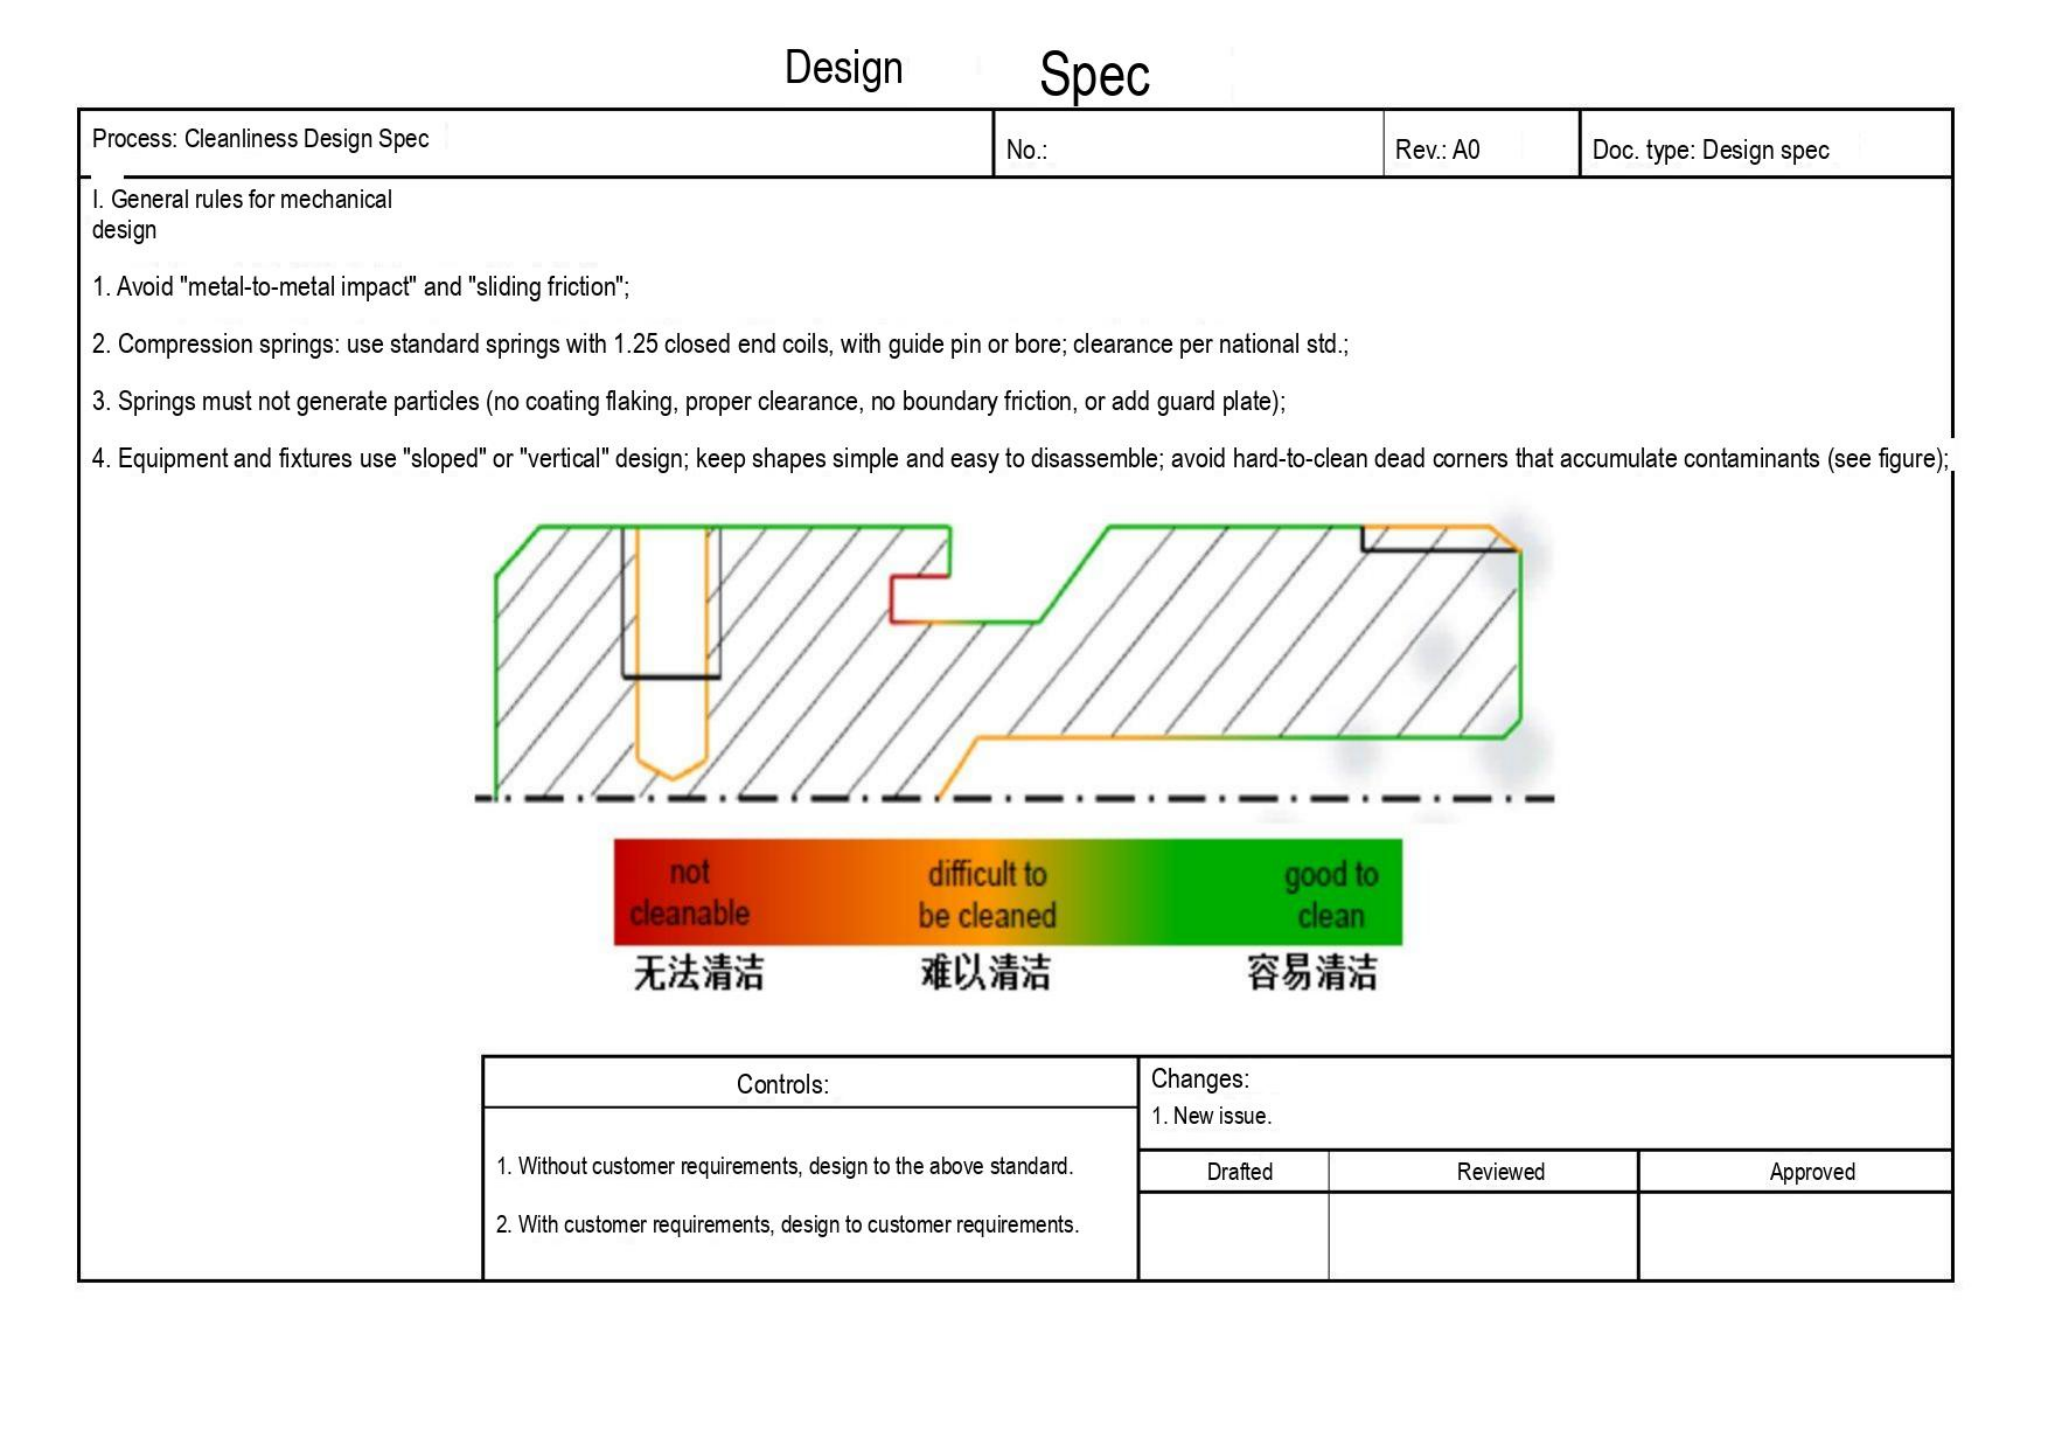Design Spec

| Process: Cleanliness Design Spec | No.: | Rev.: A0 | Doc. type: Design spec |
|---|---|---|---|

I. General rules for mechanical design

1. Avoid "metal-to-metal impact" and "sliding friction";

2. Compression springs: use standard springs with 1.25 closed end coils, with guide pin or bore; clearance per national std.;

3. Springs must not generate particles (no coating flaking, proper clearance, no boundary friction, or add guard plate);

4. Equipment and fixtures use "sloped" or "vertical" design; keep shapes simple and easy to disassemble; avoid hard-to-clean dead corners that accumulate contaminants (see figure);

not cleanable
无法清洁

difficult to be cleaned
难以清洁

good to clean
容易清洁

| Controls: |
|---|
| 1. Without customer requirements, design to the above standard.<br>2. With customer requirements, design to customer requirements. |

Changes:
1. New issue.

| Drafted | Reviewed | Approved |
|---|---|---|
| | | |
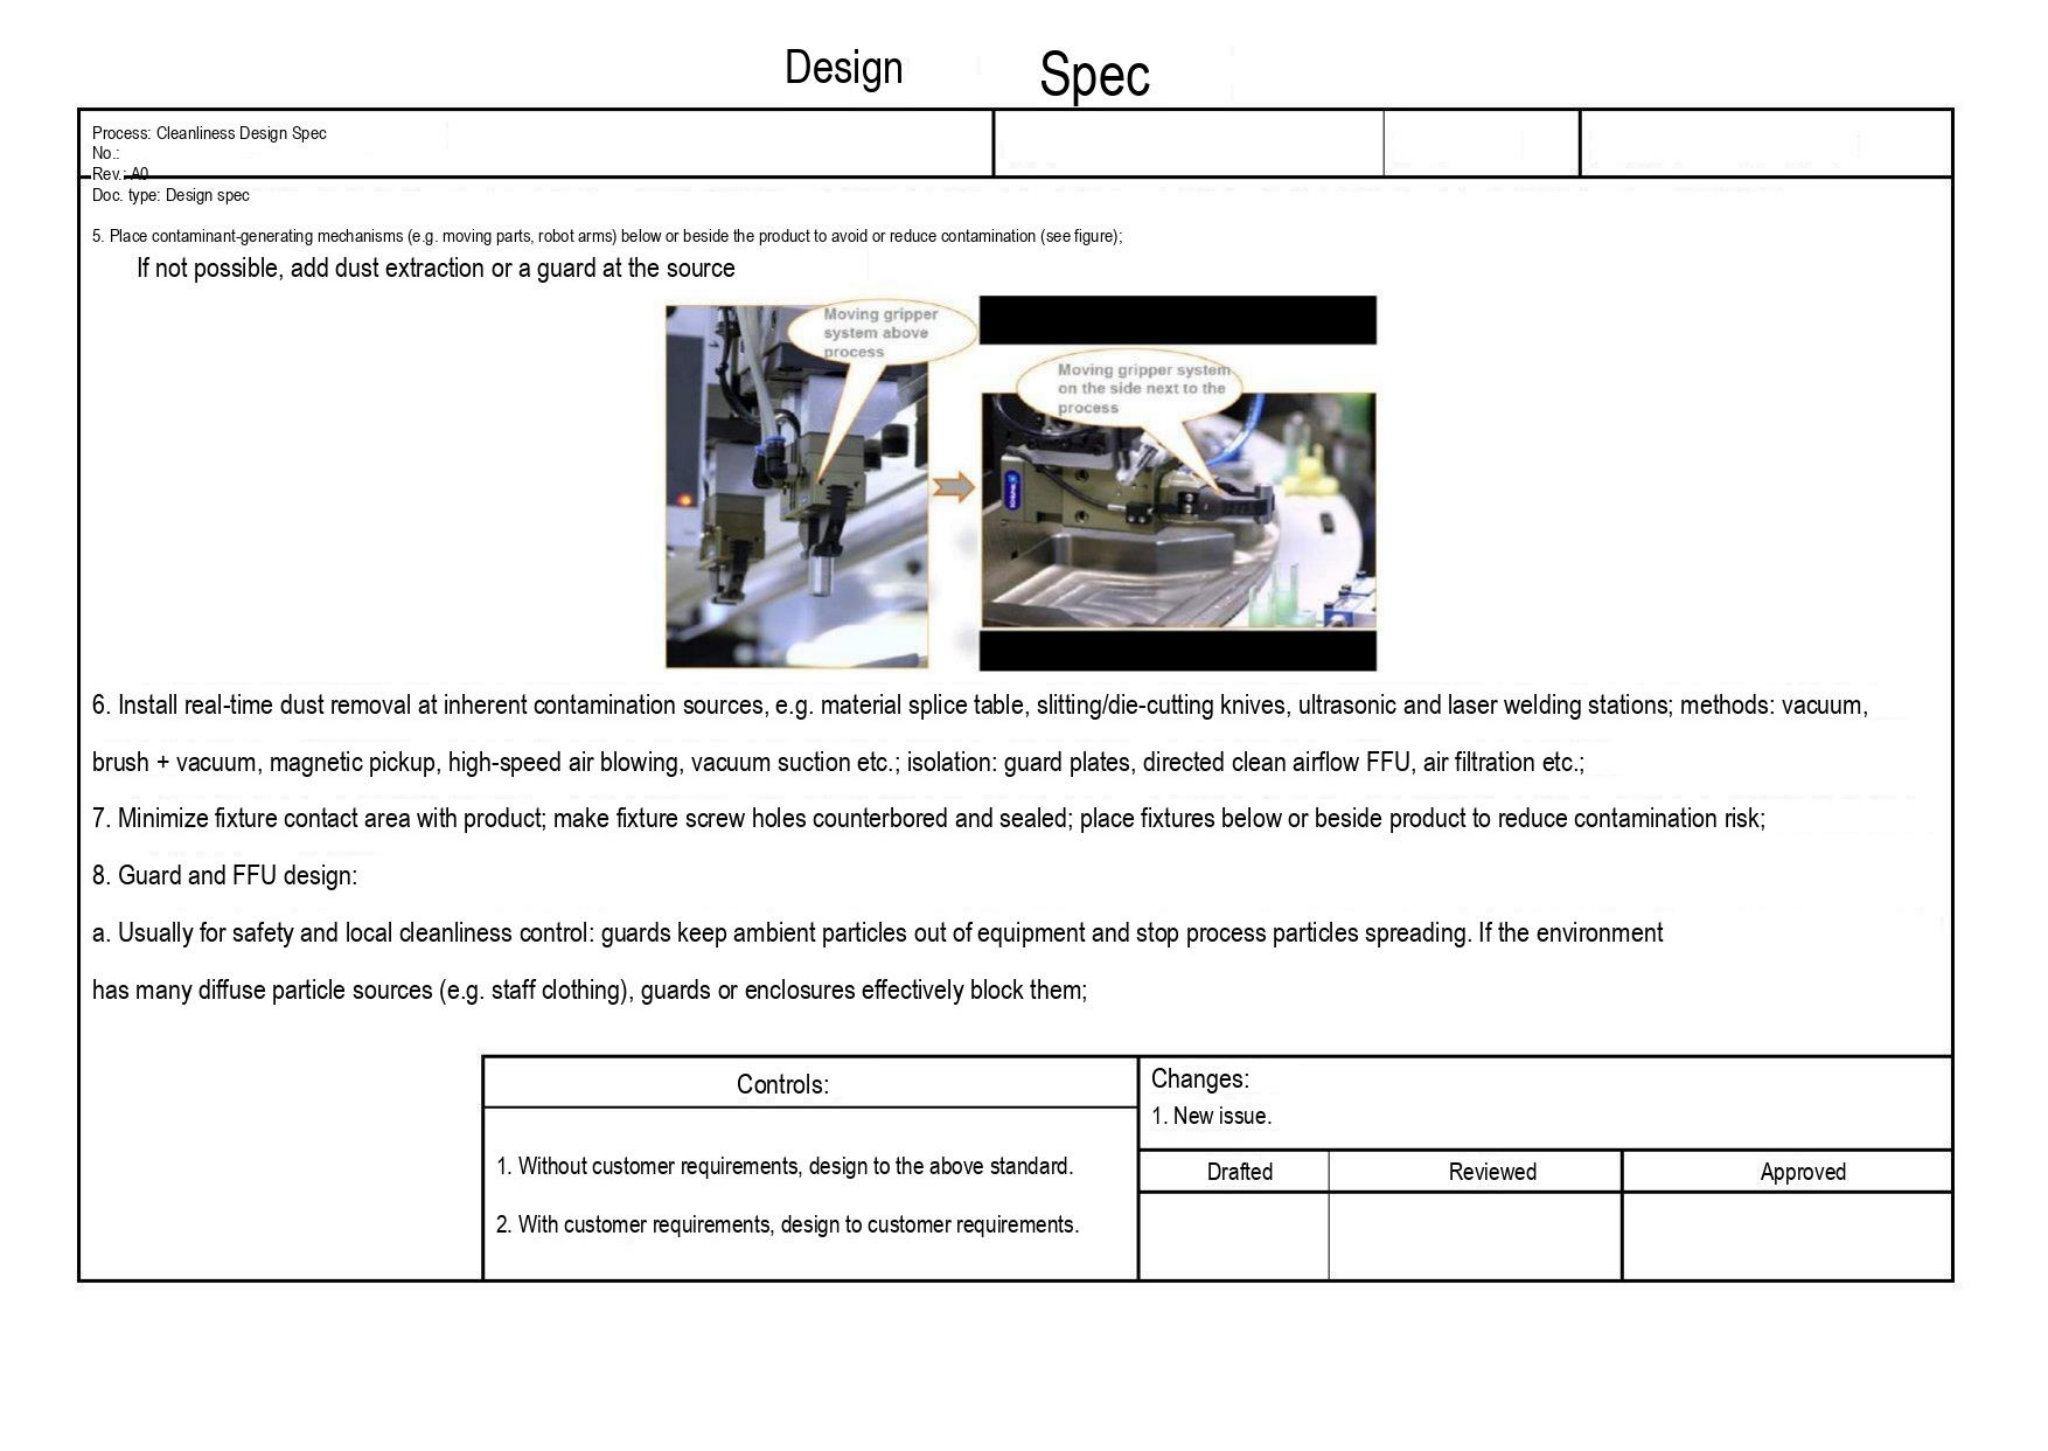Design Spec

Process: Cleanliness Design Spec
No.:
Rev.: A0
Doc. type: Design spec

5. Place contaminant-generating mechanisms (e.g. moving parts, robot arms) below or beside the product to avoid or reduce contamination (see figure);
If not possible, add dust extraction or a guard at the source

Moving gripper system above process

Moving gripper system on the side next to the process

6. Install real-time dust removal at inherent contamination sources, e.g. material splice table, slitting/die-cutting knives, ultrasonic and laser welding stations; methods: vacuum, brush + vacuum, magnetic pickup, high-speed air blowing, vacuum suction etc.; isolation: guard plates, directed clean airflow FFU, air filtration etc.;

7. Minimize fixture contact area with product; make fixture screw holes counterbored and sealed; place fixtures below or beside product to reduce contamination risk;

8. Guard and FFU design:

a. Usually for safety and local cleanliness control: guards keep ambient particles out of equipment and stop process particles spreading. If the environment has many diffuse particle sources (e.g. staff clothing), guards or enclosures effectively block them;

| Controls: |
|---|
| 1. Without customer requirements, design to the above standard.<br>2. With customer requirements, design to customer requirements. |

Changes:
1. New issue.

| Drafted | Reviewed | Approved |
|---|---|---|
| | | |
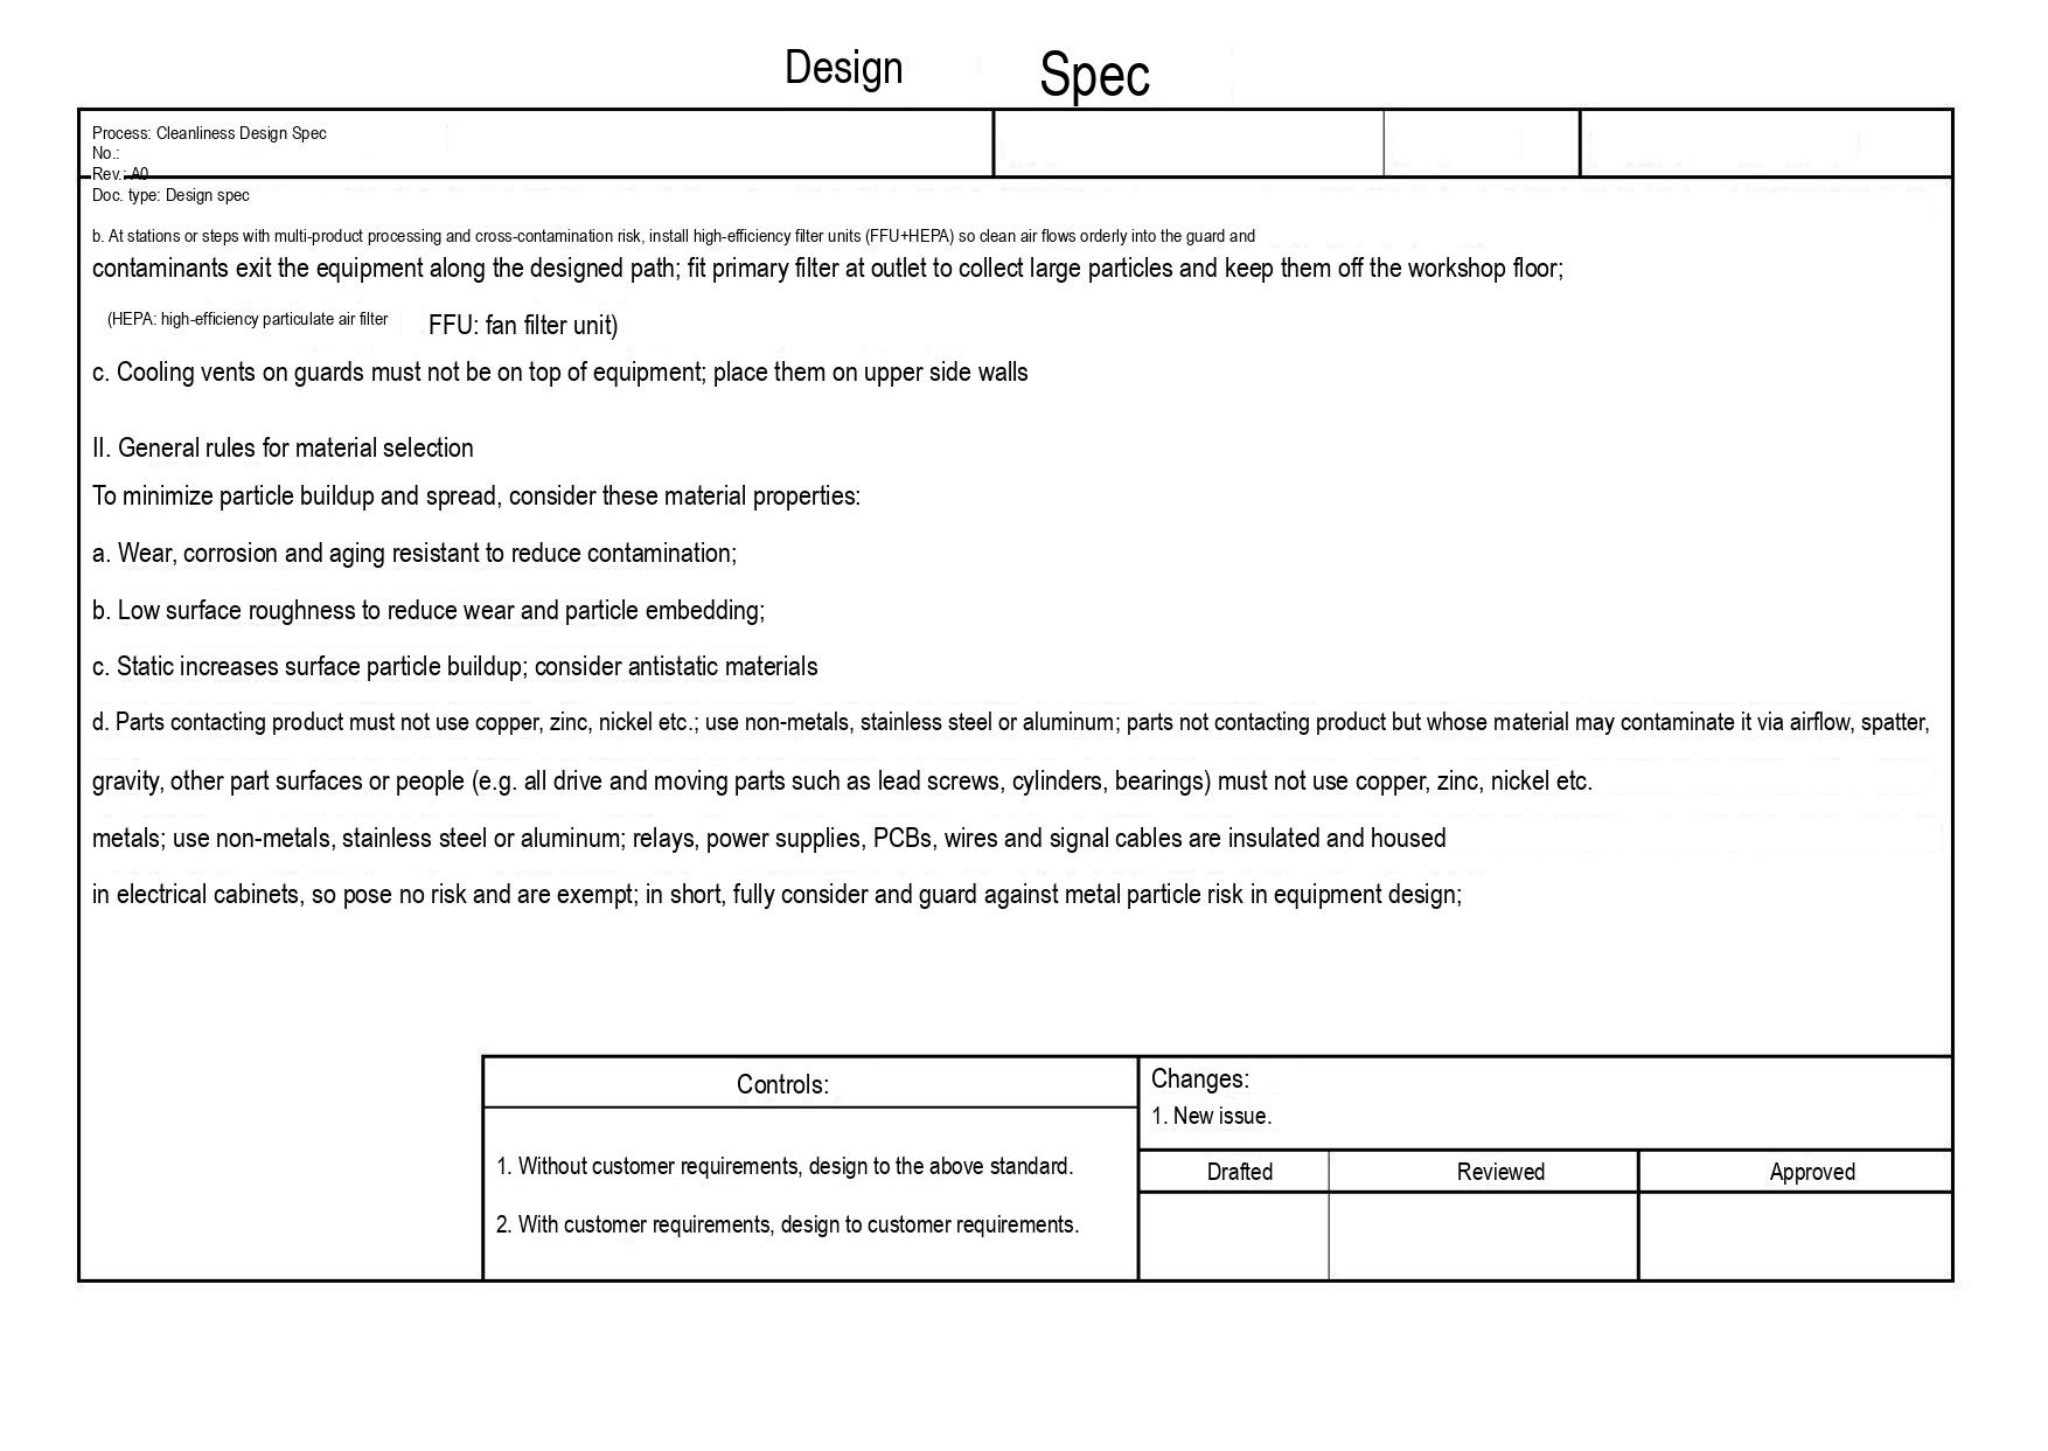Design Spec

Process: Cleanliness Design Spec
No.:
Rev.: A0
Doc. type: Design spec

b. At stations or steps with multi-product processing and cross-contamination risk, install high-efficiency filter units (FFU+HEPA) so clean air flows orderly into the guard and contaminants exit the equipment along the designed path; fit primary filter at outlet to collect large particles and keep them off the workshop floor;

(HEPA: high-efficiency particulate air filter FFU: fan filter unit)

c. Cooling vents on guards must not be on top of equipment; place them on upper side walls

II. General rules for material selection

To minimize particle buildup and spread, consider these material properties:

a. Wear, corrosion and aging resistant to reduce contamination;

b. Low surface roughness to reduce wear and particle embedding;

c. Static increases surface particle buildup; consider antistatic materials

d. Parts contacting product must not use copper, zinc, nickel etc.; use non-metals, stainless steel or aluminum; parts not contacting product but whose material may contaminate it via airflow, spatter, gravity, other part surfaces or people (e.g. all drive and moving parts such as lead screws, cylinders, bearings) must not use copper, zinc, nickel etc. metals; use non-metals, stainless steel or aluminum; relays, power supplies, PCBs, wires and signal cables are insulated and housed in electrical cabinets, so pose no risk and are exempt; in short, fully consider and guard against metal particle risk in equipment design;

| Controls: | Changes: |
|---|---|
| 1. Without customer requirements, design to the above standard. <br> 2. With customer requirements, design to customer requirements. | 1. New issue. |

| Drafted | Reviewed | Approved |
|---|---|---|
| | | |
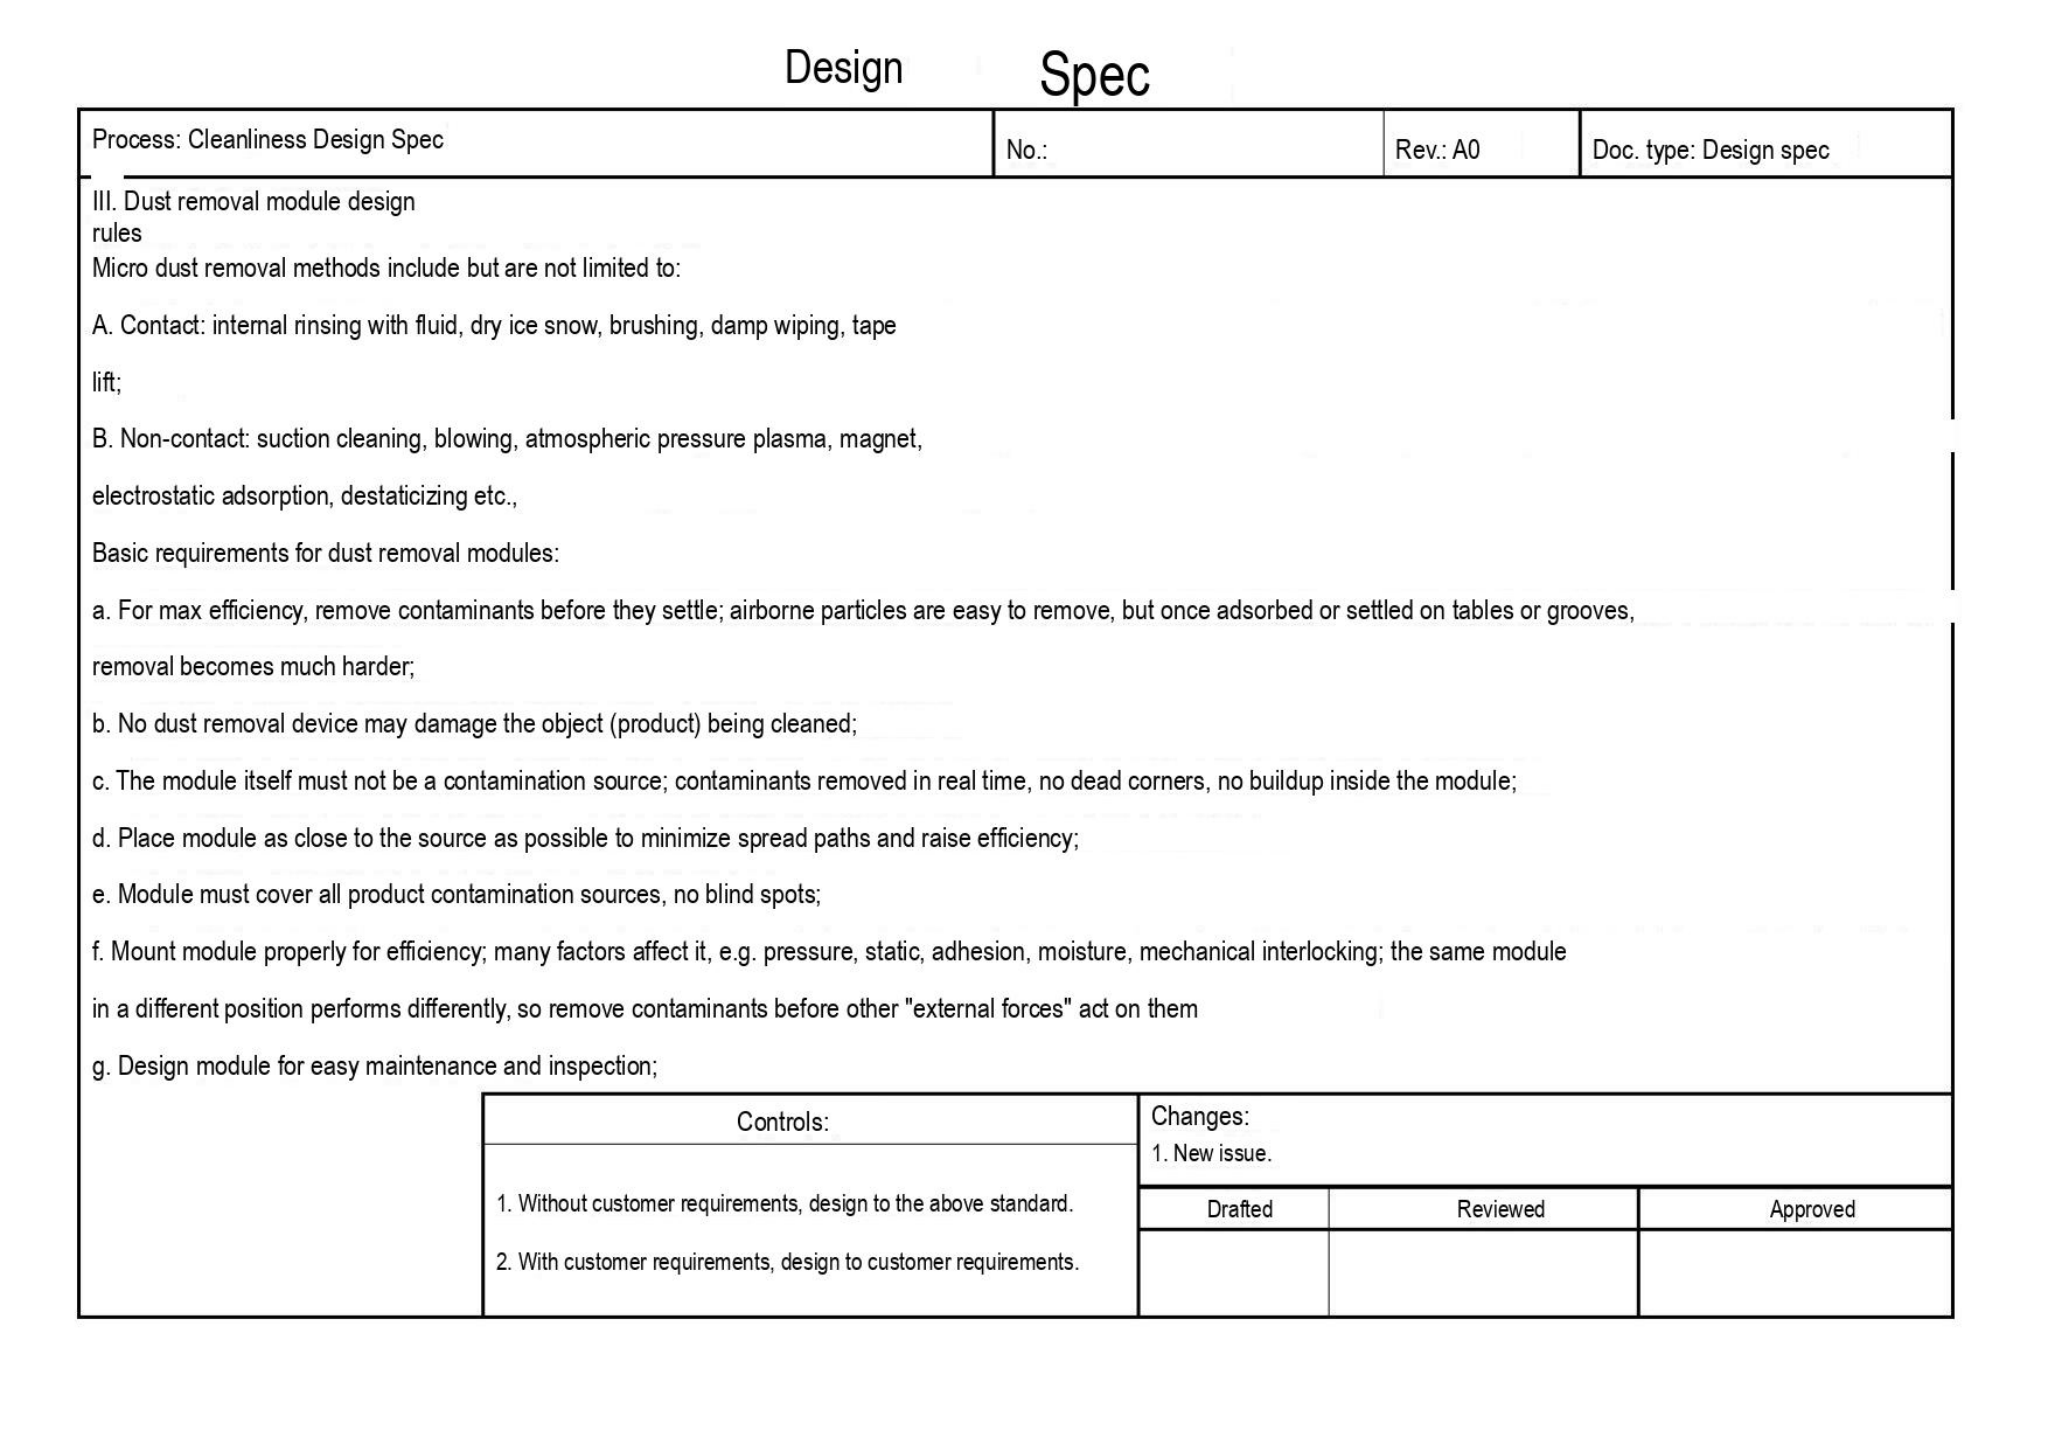Design Spec

| Process: Cleanliness Design Spec | No.: | Rev.: A0 | Doc. type: Design spec |
|---|---|---|---|

III. Dust removal module design
rules
Micro dust removal methods include but are not limited to:

A. Contact: internal rinsing with fluid, dry ice snow, brushing, damp wiping, tape

lift;

B. Non-contact: suction cleaning, blowing, atmospheric pressure plasma, magnet,

electrostatic adsorption, destaticizing etc.,

Basic requirements for dust removal modules:

a. For max efficiency, remove contaminants before they settle; airborne particles are easy to remove, but once adsorbed or settled on tables or grooves,

removal becomes much harder;

b. No dust removal device may damage the object (product) being cleaned;

c. The module itself must not be a contamination source; contaminants removed in real time, no dead corners, no buildup inside the module;

d. Place module as close to the source as possible to minimize spread paths and raise efficiency;

e. Module must cover all product contamination sources, no blind spots;

f. Mount module properly for efficiency; many factors affect it, e.g. pressure, static, adhesion, moisture, mechanical interlocking; the same module

in a different position performs differently, so remove contaminants before other "external forces" act on them

g. Design module for easy maintenance and inspection;

| Controls: |
|---|
| 1. Without customer requirements, design to the above standard.<br><br>2. With customer requirements, design to customer requirements. |

Changes:
1. New issue.

| Drafted | Reviewed | Approved |
|---|---|---|
| | | |
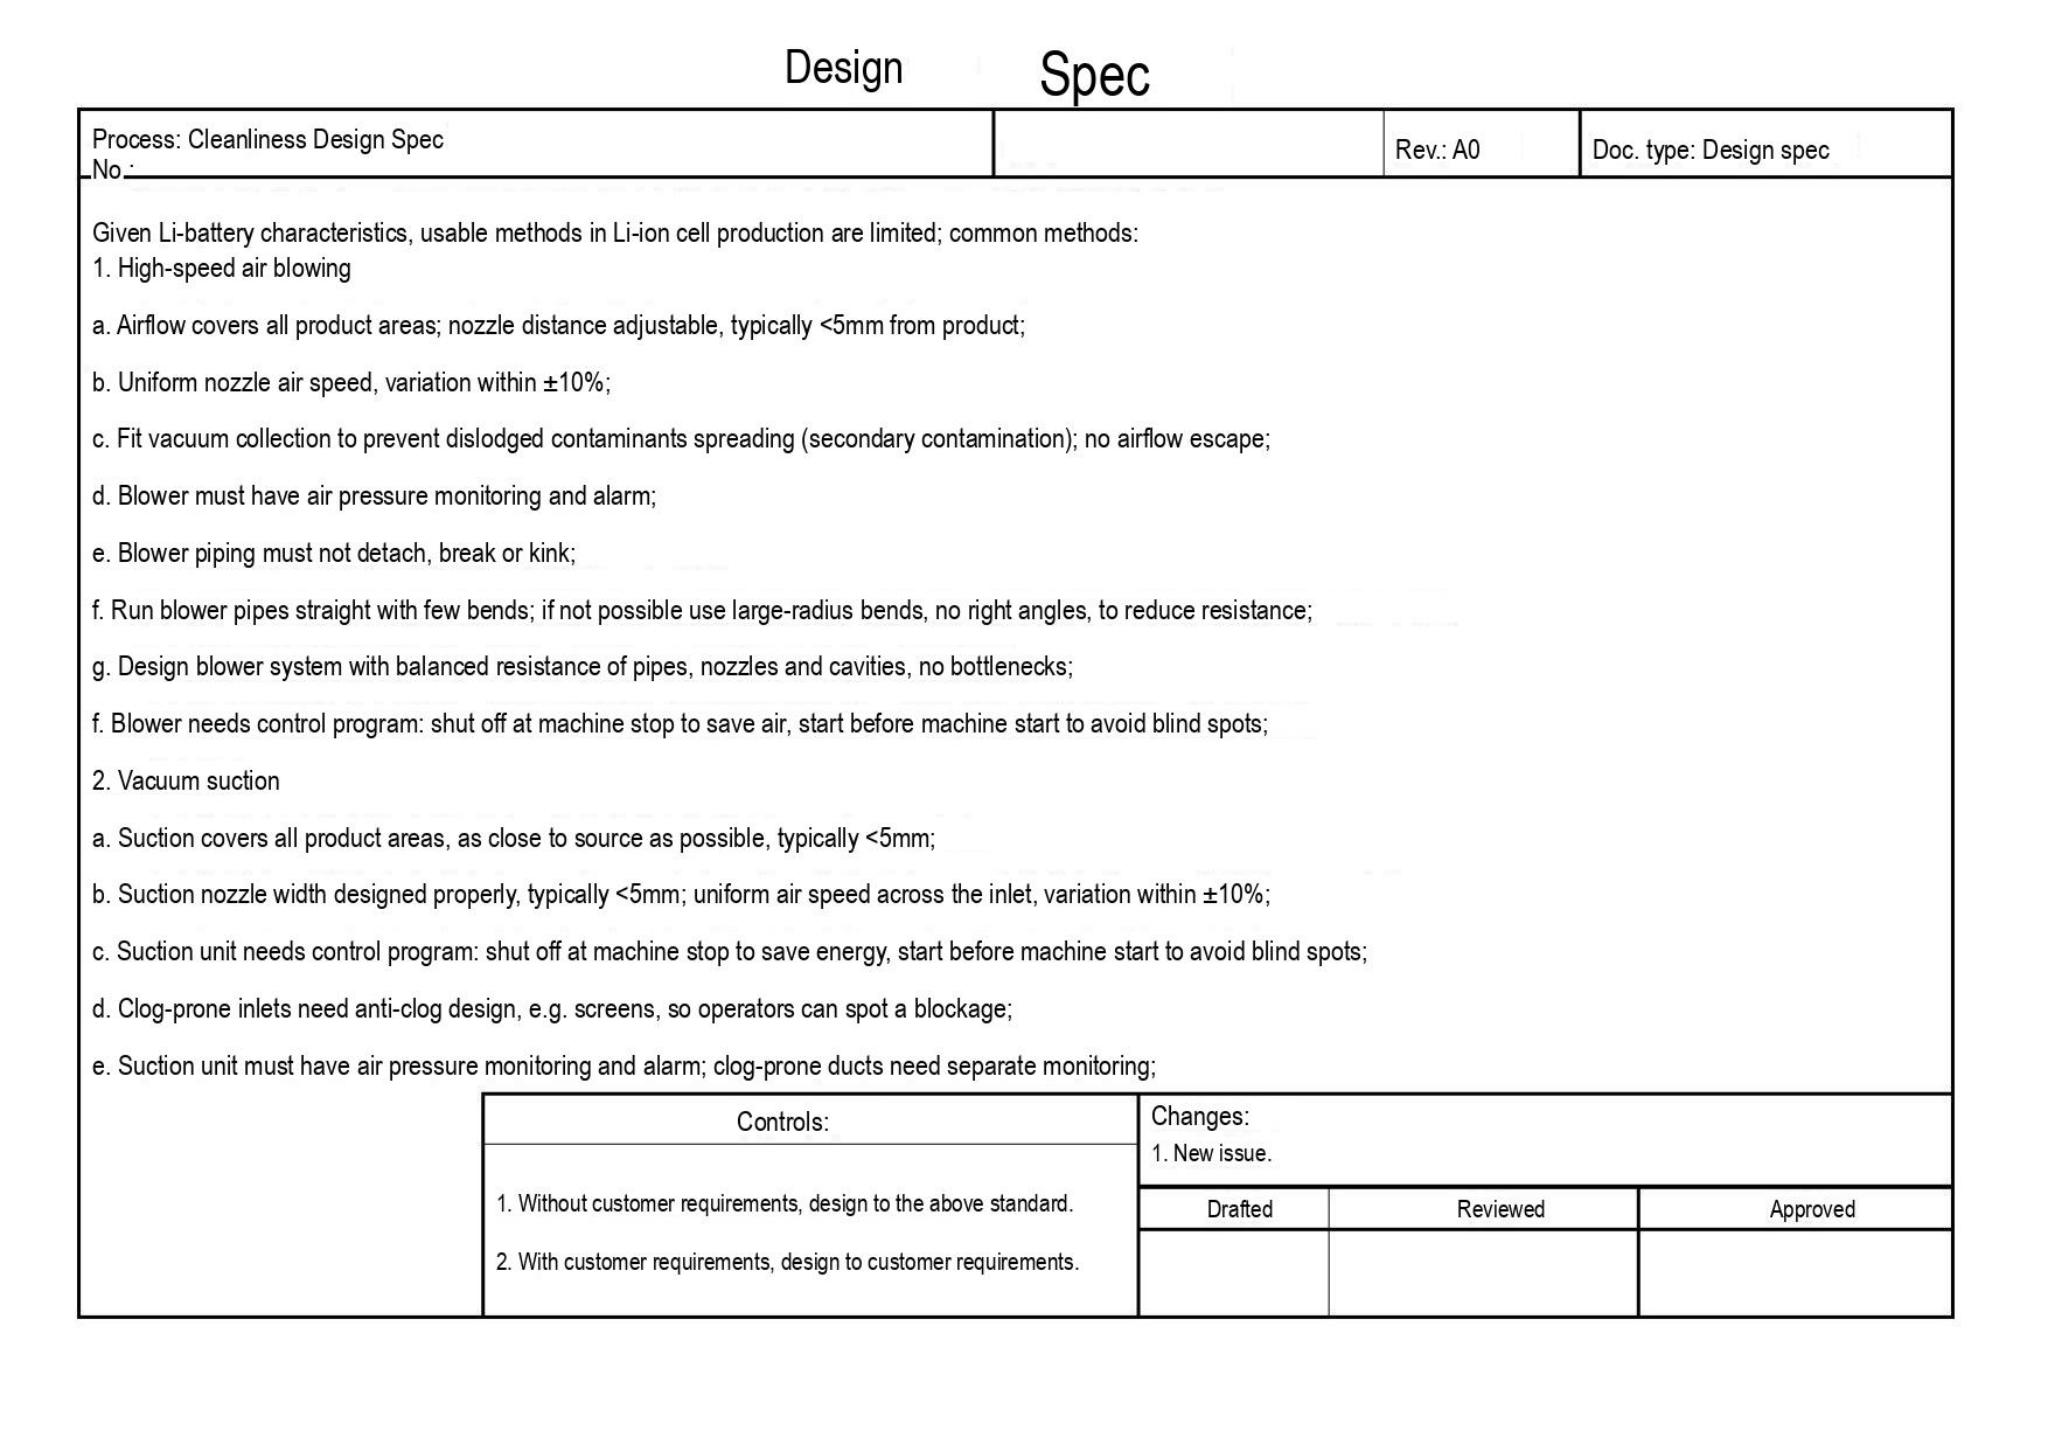Design Spec

| Process: Cleanliness Design Spec<br>No.: | | Rev.: A0 | Doc. type: Design spec |
|---|---|---|---|

Given Li-battery characteristics, usable methods in Li-ion cell production are limited; common methods:
1. High-speed air blowing

a. Airflow covers all product areas; nozzle distance adjustable, typically <5mm from product;

b. Uniform nozzle air speed, variation within ±10%;

c. Fit vacuum collection to prevent dislodged contaminants spreading (secondary contamination); no airflow escape;

d. Blower must have air pressure monitoring and alarm;

e. Blower piping must not detach, break or kink;

f. Run blower pipes straight with few bends; if not possible use large-radius bends, no right angles, to reduce resistance;

g. Design blower system with balanced resistance of pipes, nozzles and cavities, no bottlenecks;

f. Blower needs control program: shut off at machine stop to save air, start before machine start to avoid blind spots;

2. Vacuum suction

a. Suction covers all product areas, as close to source as possible, typically <5mm;

b. Suction nozzle width designed properly, typically <5mm; uniform air speed across the inlet, variation within ±10%;

c. Suction unit needs control program: shut off at machine stop to save energy, start before machine start to avoid blind spots;

d. Clog-prone inlets need anti-clog design, e.g. screens, so operators can spot a blockage;

e. Suction unit must have air pressure monitoring and alarm; clog-prone ducts need separate monitoring;

| Controls: | Changes:<br>1. New issue. | | |
|---|---|---|---|
| 1. Without customer requirements, design to the above standard.<br><br>2. With customer requirements, design to customer requirements. | Drafted | Reviewed | Approved |
| | | | |
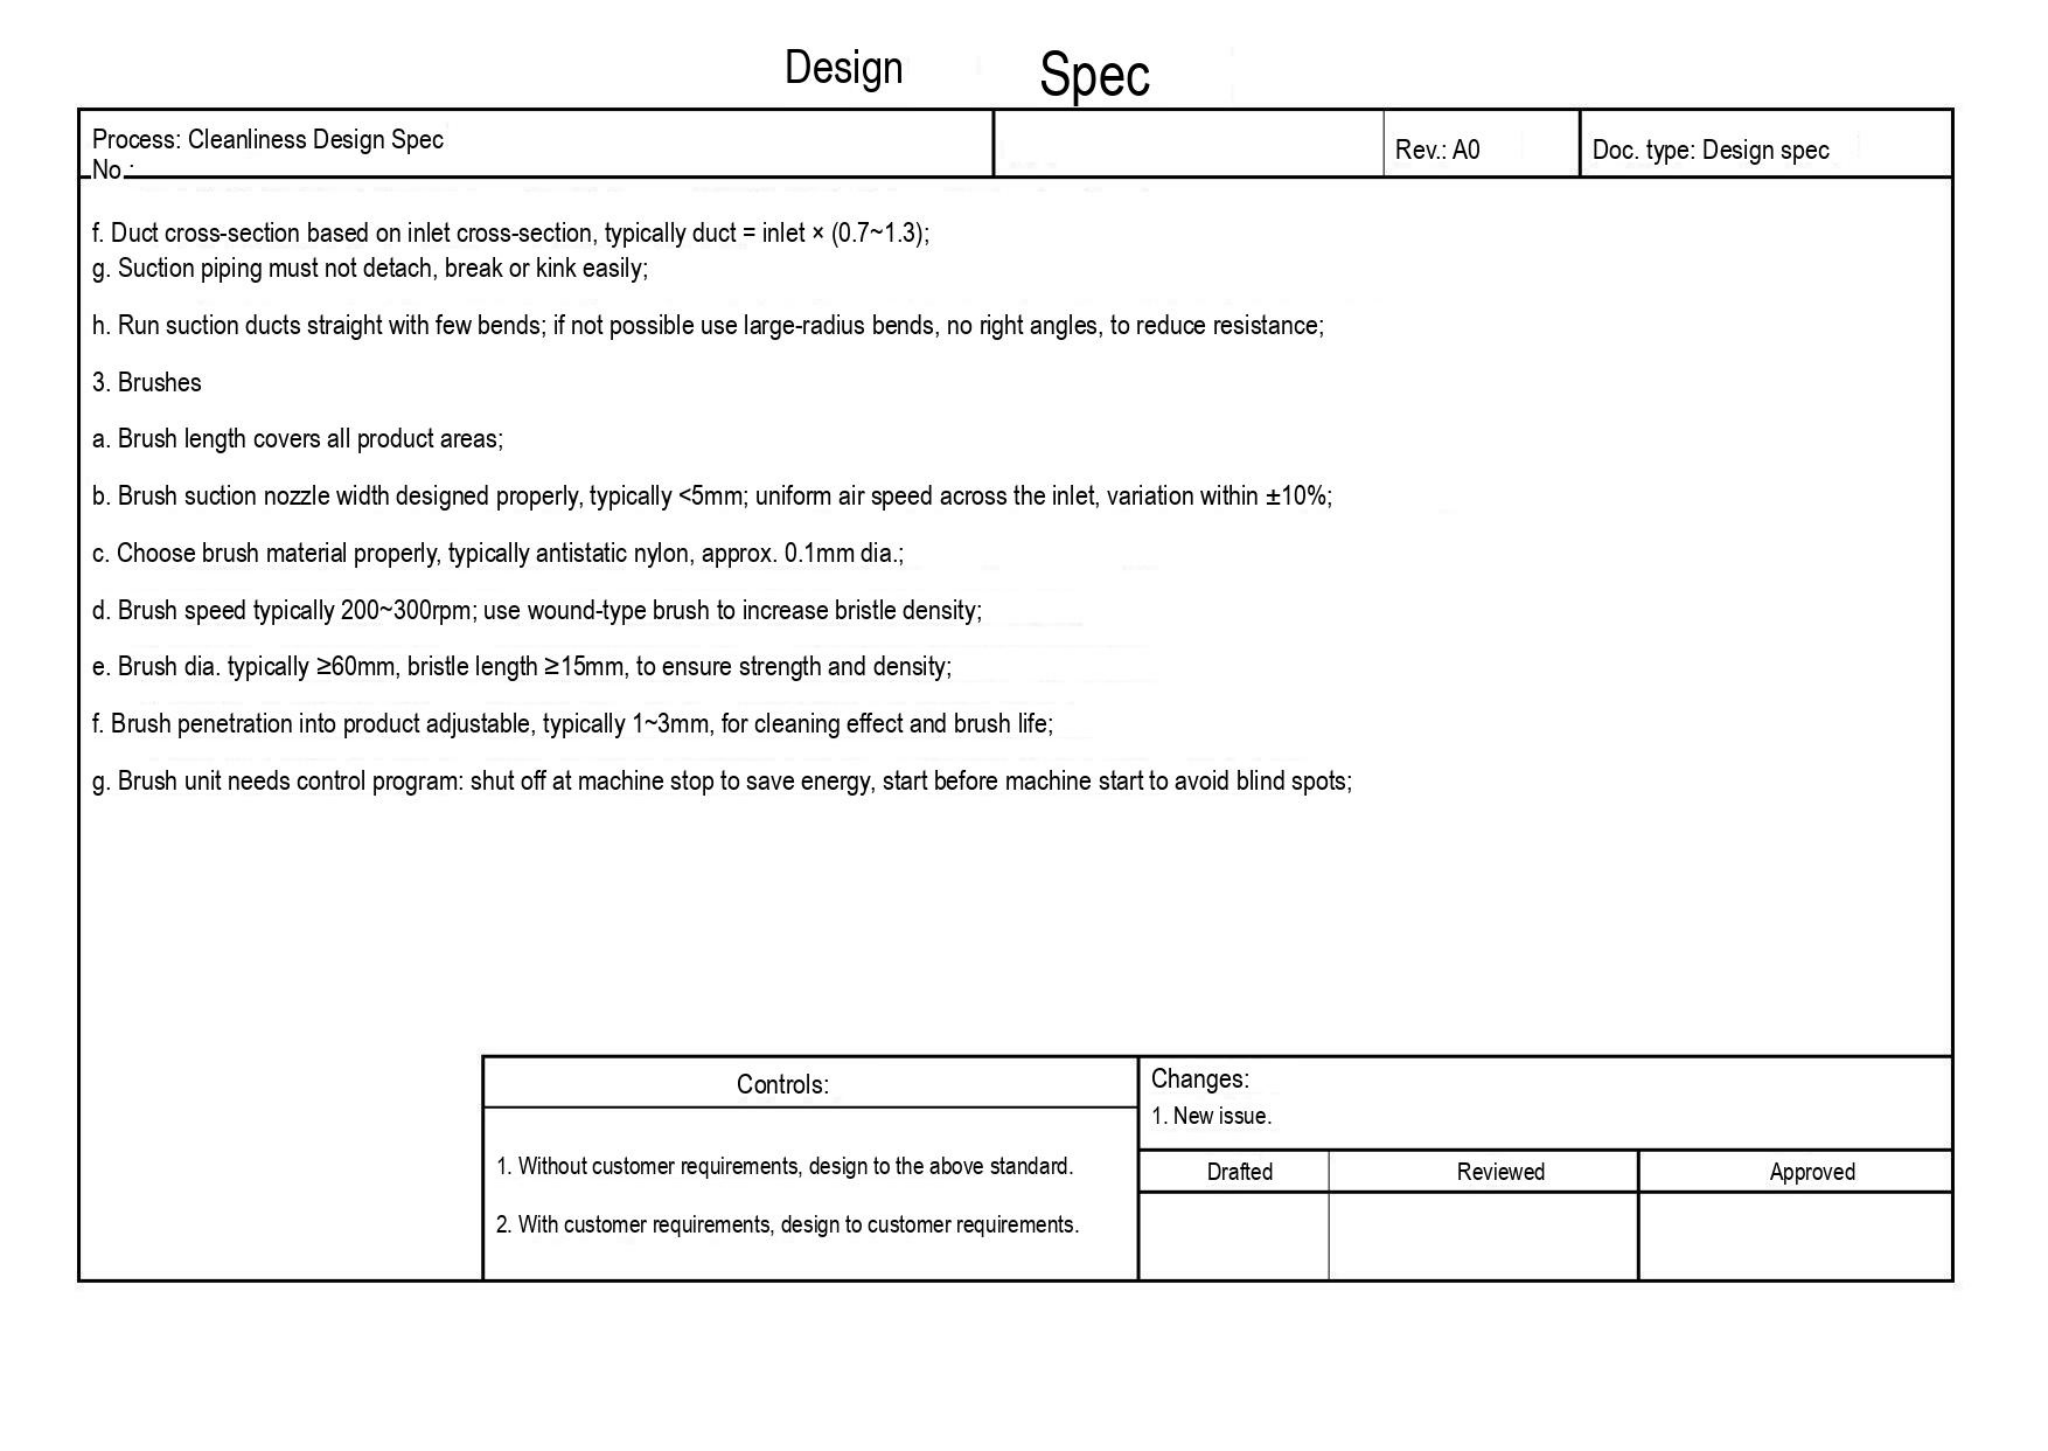Design Spec

| Process: Cleanliness Design Spec<br>No.: | | Rev.: A0 | Doc. type: Design spec |
|---|---|---|---|

f. Duct cross-section based on inlet cross-section, typically duct = inlet × (0.7~1.3);
g. Suction piping must not detach, break or kink easily;

h. Run suction ducts straight with few bends; if not possible use large-radius bends, no right angles, to reduce resistance;

3. Brushes

a. Brush length covers all product areas;

b. Brush suction nozzle width designed properly, typically <5mm; uniform air speed across the inlet, variation within ±10%;

c. Choose brush material properly, typically antistatic nylon, approx. 0.1mm dia.;

d. Brush speed typically 200~300rpm; use wound-type brush to increase bristle density;

e. Brush dia. typically ≥60mm, bristle length ≥15mm, to ensure strength and density;

f. Brush penetration into product adjustable, typically 1~3mm, for cleaning effect and brush life;

g. Brush unit needs control program: shut off at machine stop to save energy, start before machine start to avoid blind spots;

| Controls: |
|---|
| 1. Without customer requirements, design to the above standard.<br>2. With customer requirements, design to customer requirements. |

Changes:
1. New issue.

| Drafted | Reviewed | Approved |
|---|---|---|
| | | |